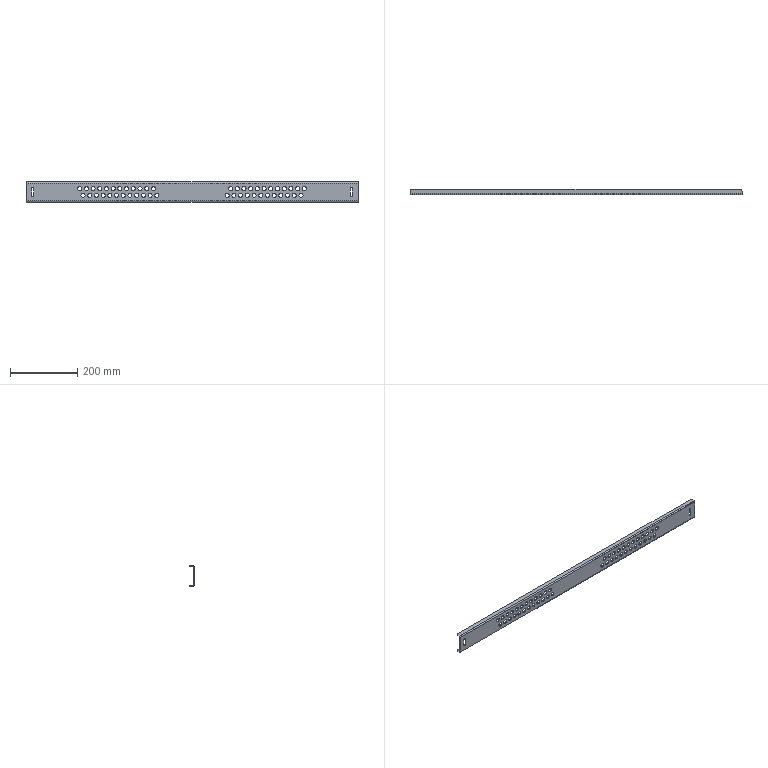Part | SolidWorks | features ICE 3, LPattern 2, MirrorPattern 2, EdgeFlange 1, Fillet 1, FlatPattern 1, HoleWzd 1, SMBaseFlange 1, SheetMetal 1 | 1 solid | 132 faces | box 990 x 15 x 60 mm | volume 154443 mm3 | cylinder 110 | plane 22 | commonest cylinder face diameters 12.2 x96 7 x6 10 x4 2.54 x2 6.54 x2